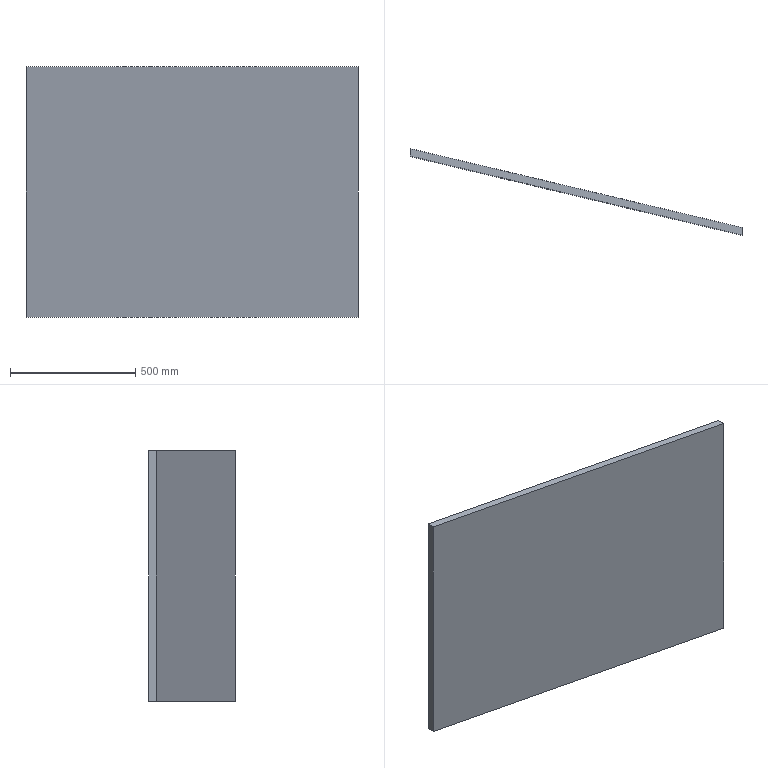Part | SolidWorks | features Extrusion 1 | 1 solid | 6 faces | box 1325 x 345 x 1000 mm | volume 39735000 mm3 | plane 6
STEP:
#1=CARTESIAN_POINT('',(0.,0.,0.));
#2=VERTEX_POINT('',#1);
#3=CARTESIAN_POINT('',(0.,-30.,0.));
#4=VERTEX_POINT('',#3);
#5=CARTESIAN_POINT('',(0.,-30.,0.));
#6=DIRECTION('',(0.,-1.,0.));
#7=VECTOR('',#6,1000.);
#8=LINE('',#5,#7);
#9=EDGE_CURVE('',#2,#4,#8,.T.);
#10=ORIENTED_EDGE('',*,*,#9,.T.);
#11=CARTESIAN_POINT('',(0.,-30.,1000.));
#12=VERTEX_POINT('',#11);
#13=CARTESIAN_POINT('',(0.,-30.,1000.));
#14=DIRECTION('',(0.,0.,-1.));
#15=VECTOR('',#14,1000.);
#16=LINE('',#13,#15);
#17=EDGE_CURVE('',#12,#4,#16,.T.);
#18=ORIENTED_EDGE('',*,*,#17,.F.);
#19=CARTESIAN_POINT('',(0.,0.,1000.));
#20=VERTEX_POINT('',#19);
#21=CARTESIAN_POINT('',(0.,-30.,1000.));
#22=DIRECTION('',(0.,-1.,0.));
#23=VECTOR('',#22,1000.);
#24=LINE('',#21,#23);
#25=EDGE_CURVE('',#20,#12,#24,.T.);
#26=ORIENTED_EDGE('',*,*,#25,.F.);
#27=CARTESIAN_POINT('',(0.,0.,1000.));
#28=DIRECTION('',(0.,0.,-1.));
#29=VECTOR('',#28,1000.);
#30=LINE('',#27,#29);
#31=EDGE_CURVE('',#20,#2,#30,.T.);
#32=ORIENTED_EDGE('',*,*,#31,.T.);
#33=EDGE_LOOP('',(#10,#18,#26,#32));
#34=FACE_OUTER_BOUND('',#33,.T.);
#35=CARTESIAN_POINT('',(0.,-30.,1000.));
#36=DIRECTION('',(1.,0.,0.));
#37=DIRECTION('',(0.,1.,0.));
#38=AXIS2_PLACEMENT_3D('',#35,#36,#37);
#39=PLANE('',#38);
#40=ADVANCED_FACE('',(#34),#39,.F.);
#41=CARTESIAN_POINT('',(1324.5,-345.,0.));
#42=VERTEX_POINT('',#41);
#43=CARTESIAN_POINT('',(1324.5,-345.,0.));
#44=DIRECTION('',(0.9729,-0.2314,0.));
#45=VECTOR('',#44,1000.);
#46=LINE('',#43,#45);
#47=EDGE_CURVE('',#4,#42,#46,.T.);
#48=ORIENTED_EDGE('',*,*,#47,.T.);
#49=CARTESIAN_POINT('',(1324.5,-345.,1000.));
#50=VERTEX_POINT('',#49);
#51=CARTESIAN_POINT('',(1324.5,-345.,1000.));
#52=DIRECTION('',(0.,0.,-1.));
#53=VECTOR('',#52,1000.);
#54=LINE('',#51,#53);
#55=EDGE_CURVE('',#50,#42,#54,.T.);
#56=ORIENTED_EDGE('',*,*,#55,.F.);
#57=CARTESIAN_POINT('',(1324.5,-345.,1000.));
#58=DIRECTION('',(0.9729,-0.2314,0.));
#59=VECTOR('',#58,1000.);
#60=LINE('',#57,#59);
#61=EDGE_CURVE('',#12,#50,#60,.T.);
#62=ORIENTED_EDGE('',*,*,#61,.F.);
#63=ORIENTED_EDGE('',*,*,#17,.T.);
#64=EDGE_LOOP('',(#48,#56,#62,#63));
#65=FACE_OUTER_BOUND('',#64,.T.);
#66=CARTESIAN_POINT('',(1324.5,-345.,1000.));
#67=DIRECTION('',(0.2314,0.9729,0.));
#68=DIRECTION('',(-0.9729,0.2314,0.));
#69=AXIS2_PLACEMENT_3D('',#66,#67,#68);
#70=PLANE('',#69);
#71=ADVANCED_FACE('',(#65),#70,.F.);
#72=CARTESIAN_POINT('',(1324.5,-315.,0.));
#73=VERTEX_POINT('',#72);
#74=CARTESIAN_POINT('',(1324.5,-315.,0.));
#75=DIRECTION('',(0.,1.,0.));
#76=VECTOR('',#75,1000.);
#77=LINE('',#74,#76);
#78=EDGE_CURVE('',#42,#73,#77,.T.);
#79=ORIENTED_EDGE('',*,*,#78,.T.);
#80=CARTESIAN_POINT('',(1324.5,-315.,1000.));
#81=VERTEX_POINT('',#80);
#82=CARTESIAN_POINT('',(1324.5,-315.,1000.));
#83=DIRECTION('',(0.,0.,-1.));
#84=VECTOR('',#83,1000.);
#85=LINE('',#82,#84);
#86=EDGE_CURVE('',#81,#73,#85,.T.);
#87=ORIENTED_EDGE('',*,*,#86,.F.);
#88=CARTESIAN_POINT('',(1324.5,-315.,1000.));
#89=DIRECTION('',(0.,1.,0.));
#90=VECTOR('',#89,1000.);
#91=LINE('',#88,#90);
#92=EDGE_CURVE('',#50,#81,#91,.T.);
#93=ORIENTED_EDGE('',*,*,#92,.F.);
#94=ORIENTED_EDGE('',*,*,#55,.T.);
#95=EDGE_LOOP('',(#79,#87,#93,#94));
#96=FACE_OUTER_BOUND('',#95,.T.);
#97=CARTESIAN_POINT('',(1324.5,-315.,1000.));
#98=DIRECTION('',(-1.,0.,0.));
#99=DIRECTION('',(0.,0.,1.));
#100=AXIS2_PLACEMENT_3D('',#97,#98,#99);
#101=PLANE('',#100);
#102=ADVANCED_FACE('',(#96),#101,.F.);
#103=CARTESIAN_POINT('',(0.,0.,0.));
#104=DIRECTION('',(-0.9729,0.2314,0.));
#105=VECTOR('',#104,1000.);
#106=LINE('',#103,#105);
#107=EDGE_CURVE('',#73,#2,#106,.T.);
#108=ORIENTED_EDGE('',*,*,#107,.T.);
#109=ORIENTED_EDGE('',*,*,#31,.F.);
#110=CARTESIAN_POINT('',(0.,0.,1000.));
#111=DIRECTION('',(-0.9729,0.2314,0.));
#112=VECTOR('',#111,1000.);
#113=LINE('',#110,#112);
#114=EDGE_CURVE('',#81,#20,#113,.T.);
#115=ORIENTED_EDGE('',*,*,#114,.F.);
#116=ORIENTED_EDGE('',*,*,#86,.T.);
#117=EDGE_LOOP('',(#108,#109,#115,#116));
#118=FACE_OUTER_BOUND('',#117,.T.);
#119=CARTESIAN_POINT('',(0.,0.,1000.));
#120=DIRECTION('',(-0.2314,-0.9729,0.));
#121=DIRECTION('',(0.9729,-0.2314,0.));
#122=AXIS2_PLACEMENT_3D('',#119,#120,#121);
#123=PLANE('',#122);
#124=ADVANCED_FACE('',(#118),#123,.F.);
#125=ORIENTED_EDGE('',*,*,#25,.T.);
#126=ORIENTED_EDGE('',*,*,#61,.T.);
#127=ORIENTED_EDGE('',*,*,#92,.T.);
#128=ORIENTED_EDGE('',*,*,#114,.T.);
#129=EDGE_LOOP('',(#125,#126,#127,#128));
#130=FACE_OUTER_BOUND('',#129,.T.);
#131=CARTESIAN_POINT('',(0.,0.,1000.));
#132=DIRECTION('',(0.,0.,-1.));
#133=DIRECTION('',(-1.,0.,0.));
#134=AXIS2_PLACEMENT_3D('',#131,#132,#133);
#135=PLANE('',#134);
#136=ADVANCED_FACE('',(#130),#135,.F.);
#137=ORIENTED_EDGE('',*,*,#9,.F.);
#138=ORIENTED_EDGE('',*,*,#107,.F.);
#139=ORIENTED_EDGE('',*,*,#78,.F.);
#140=ORIENTED_EDGE('',*,*,#47,.F.);
#141=EDGE_LOOP('',(#137,#138,#139,#140));
#142=FACE_OUTER_BOUND('',#141,.T.);
#143=CARTESIAN_POINT('',(0.,0.,0.));
#144=DIRECTION('',(0.,0.,-1.));
#145=DIRECTION('',(-1.,0.,0.));
#146=AXIS2_PLACEMENT_3D('',#143,#144,#145);
#147=PLANE('',#146);
#148=ADVANCED_FACE('',(#142),#147,.T.);
#149=CLOSED_SHELL('',(#40,#71,#102,#124,#136,#148));
#150=MANIFOLD_SOLID_BREP('',#149);
#151=CARTESIAN_POINT('',(0.,0.,0.));
#152=DIRECTION('',(0.,0.,1.));
#153=DIRECTION('',(1.,0.,0.));
#154=AXIS2_PLACEMENT_3D('',#151,#152,#153);
#155=(LENGTH_UNIT()NAMED_UNIT(*)SI_UNIT(.MILLI.,.METRE.));
#156=UNCERTAINTY_MEASURE_WITH_UNIT(LENGTH_MEASURE(0.00001),#155,'','');
#157=(NAMED_UNIT(*)PLANE_ANGLE_UNIT()SI_UNIT($,.RADIAN.));
#158=(NAMED_UNIT(*)SI_UNIT($,.STERADIAN.)SOLID_ANGLE_UNIT());
#159=(GEOMETRIC_REPRESENTATION_CONTEXT(3)GLOBAL_UNCERTAINTY_ASSIGNED_CONTEXT((#156))GLOBAL_UNIT_ASSIGNED_CONTEXT((#155,#157,#158))REPRESENTATION_CONTEXT('',''));
#160=ADVANCED_BREP_SHAPE_REPRESENTATION('',(#150,#154),#159);